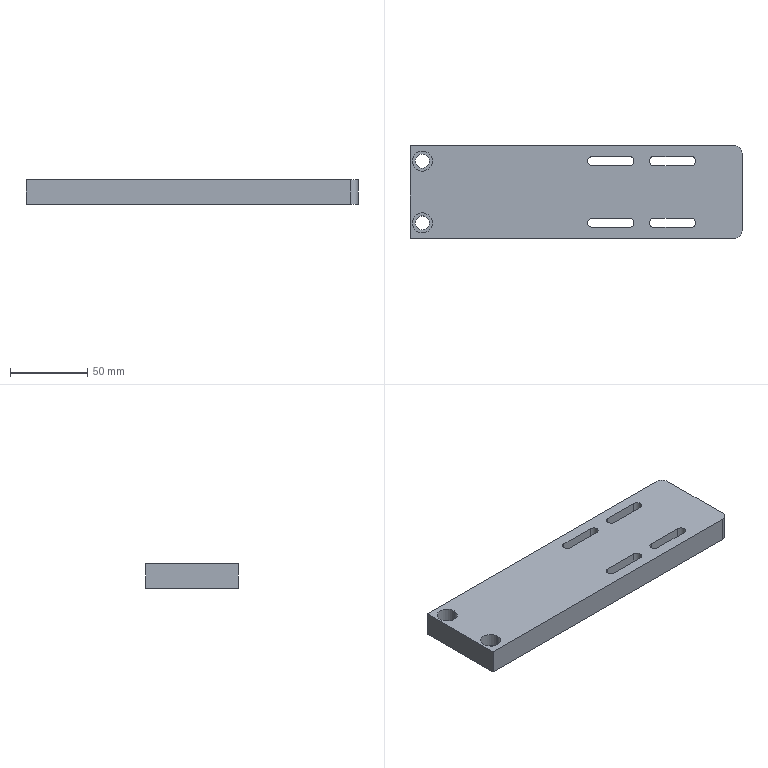NC program | Mastercam | posted with a generic post | part box 215 x 60 x 16 mm
Lines 1 to 23 of 6620:
%
O0000()
(MATERIAL - ALUMINUM MM - 2024)
( T24 | 100 FEM | H24 )
( T10 | 10 FEM | H10 | XY STOCK TO LEAVE - .15 | Z STOCK TO LEAVE - 0. )
( T7 | 6 CHM | H7 )
( T1 | 5.5 DR | H1 )
( T6 | 6 FEM | H6 )
( T5 | 5 FEM | H5 )
( T21 | 12 FEM | H21 )
N100 G21
N110 G0 G17 G40 G49 G80 G90
N120 T24 M6
N130 G0 G90 G54 X-222.5 Y0. A0. S4000 M3
N140 G43 H24 Z25. M8
N150 Z1.
N160 G1 Z0. F600.
N170 X222.5 F1000.
N180 G0 Z25.
N190 M5
N200 G91 G28 Z0. M9
N210 A0.
N220 M01